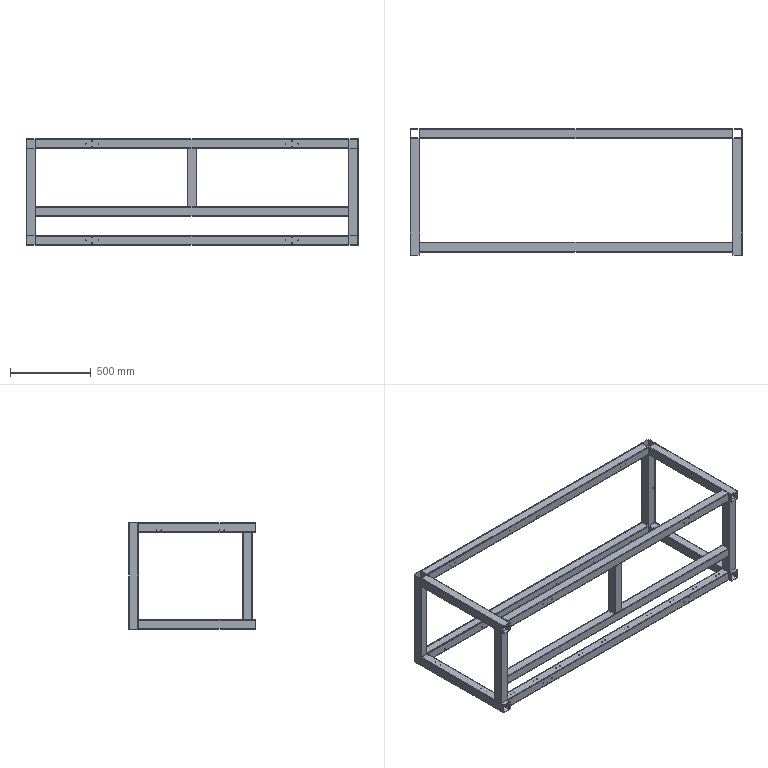Part | STEP file | JBJ-P-1011-01_Default<As Machined> | 14 solids | 372 faces | box 2060 x 785 x 660 mm | volume 6965284 mm3 | cylinder 232 | plane 140 | commonest cylinder face diameters 5 x80 4 x56 8 x56 2.5 x40